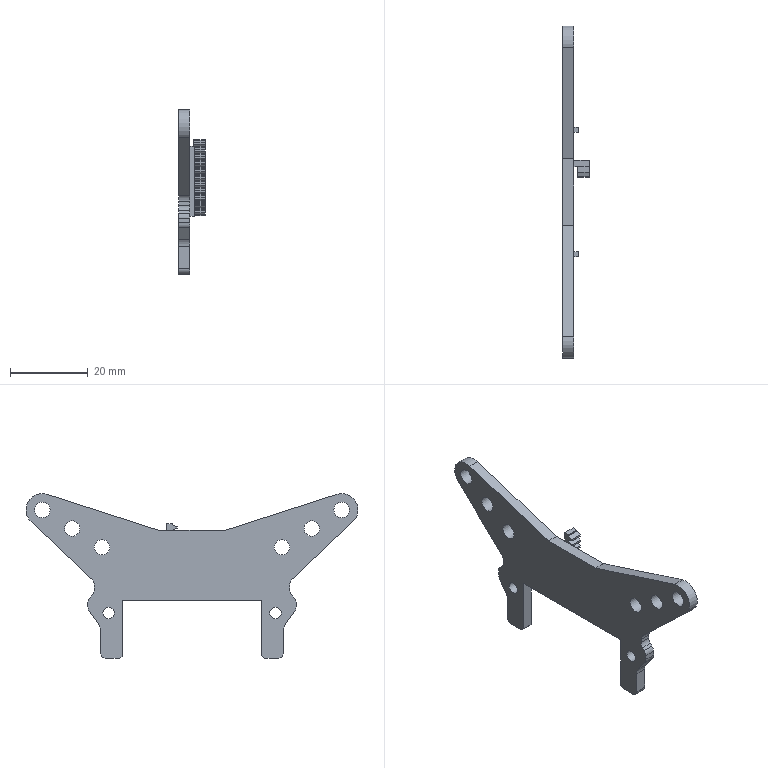Part | STEP file | Zapas-_111-007-1 | 1 solid | 154 faces | box 6.85 x 85.559 x 42.443 mm | volume 4712 mm3 | plane 85 | cylinder 69 | commonest cylinder face diameters 0.119 x22 0.199 x22 4 x14 3 x6 8.402 x3 6 x2